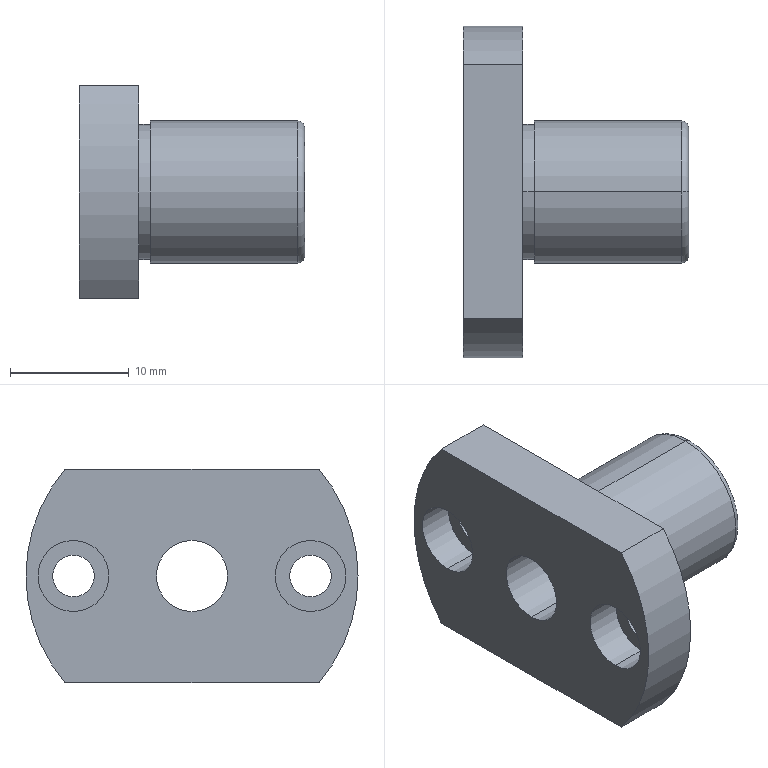Part | STEP file | 11-LHFC6C11_LHFC6 | 1 solid | 26 faces | box 19 x 28 x 18 mm | volume 3154 mm3 | cylinder 16 | plane 8 | torus 2 | commonest cylinder face diameters 6 x6 3.5 x4 11.4 x2 12 x2 28 x2
STEP:
#1=CARTESIAN_POINT('',(5.,-10.,-1.75));
#2=VERTEX_POINT('',#1);
#3=CARTESIAN_POINT('',(5.,-10.,1.75));
#4=VERTEX_POINT('',#3);
#5=CARTESIAN_POINT('',(5.,-10.,0.));
#6=DIRECTION('',(-1.,0.,0.));
#7=DIRECTION('',(0.,0.,1.));
#8=AXIS2_PLACEMENT_3D('',#5,#6,#7);
#9=CIRCLE('',#8,1.75);
#10=EDGE_CURVE('',#2,#4,#9,.T.);
#11=ORIENTED_EDGE('',*,*,#10,.F.);
#12=CARTESIAN_POINT('',(3.1,-10.,-1.75));
#13=VERTEX_POINT('',#12);
#14=CARTESIAN_POINT('',(5.,-10.,-1.75));
#15=DIRECTION('',(-1.,0.,0.));
#16=VECTOR('',#15,1000.);
#17=LINE('',#14,#16);
#18=EDGE_CURVE('',#2,#13,#17,.T.);
#19=ORIENTED_EDGE('',*,*,#18,.T.);
#20=CARTESIAN_POINT('',(3.1,-10.,1.75));
#21=VERTEX_POINT('',#20);
#22=CARTESIAN_POINT('',(3.1,-10.,0.));
#23=DIRECTION('',(-1.,0.,0.));
#24=DIRECTION('',(0.,0.,1.));
#25=AXIS2_PLACEMENT_3D('',#22,#23,#24);
#26=CIRCLE('',#25,1.75);
#27=EDGE_CURVE('',#13,#21,#26,.T.);
#28=ORIENTED_EDGE('',*,*,#27,.T.);
#29=CARTESIAN_POINT('',(5.,-10.,1.75));
#30=DIRECTION('',(-1.,0.,0.));
#31=VECTOR('',#30,1000.);
#32=LINE('',#29,#31);
#33=EDGE_CURVE('',#4,#21,#32,.T.);
#34=ORIENTED_EDGE('',*,*,#33,.F.);
#35=EDGE_LOOP('',(#11,#19,#28,#34));
#36=FACE_OUTER_BOUND('',#35,.T.);
#37=CARTESIAN_POINT('',(5.,-10.,0.));
#38=DIRECTION('',(-1.,0.,0.));
#39=DIRECTION('',(0.,0.,1.));
#40=AXIS2_PLACEMENT_3D('',#37,#38,#39);
#41=CYLINDRICAL_SURFACE('',#40,1.75);
#42=ADVANCED_FACE('',(#36),#41,.F.);
#43=CARTESIAN_POINT('',(3.1,-10.,-3.));
#44=VERTEX_POINT('',#43);
#45=CARTESIAN_POINT('',(3.1,-10.,3.));
#46=VERTEX_POINT('',#45);
#47=CARTESIAN_POINT('',(3.1,-10.,0.));
#48=DIRECTION('',(-1.,0.,0.));
#49=DIRECTION('',(0.,0.,1.));
#50=AXIS2_PLACEMENT_3D('',#47,#48,#49);
#51=CIRCLE('',#50,3.);
#52=EDGE_CURVE('',#44,#46,#51,.T.);
#53=ORIENTED_EDGE('',*,*,#52,.F.);
#54=CARTESIAN_POINT('',(0.,-10.,-3.));
#55=VERTEX_POINT('',#54);
#56=CARTESIAN_POINT('',(5.,-10.,-3.));
#57=DIRECTION('',(-1.,0.,0.));
#58=VECTOR('',#57,1000.);
#59=LINE('',#56,#58);
#60=EDGE_CURVE('',#44,#55,#59,.T.);
#61=ORIENTED_EDGE('',*,*,#60,.T.);
#62=CARTESIAN_POINT('',(0.,-10.,3.));
#63=VERTEX_POINT('',#62);
#64=CARTESIAN_POINT('',(0.,-10.,0.));
#65=DIRECTION('',(-1.,0.,0.));
#66=DIRECTION('',(0.,0.,1.));
#67=AXIS2_PLACEMENT_3D('',#64,#65,#66);
#68=CIRCLE('',#67,3.);
#69=EDGE_CURVE('',#55,#63,#68,.T.);
#70=ORIENTED_EDGE('',*,*,#69,.T.);
#71=CARTESIAN_POINT('',(5.,-10.,3.));
#72=DIRECTION('',(-1.,0.,0.));
#73=VECTOR('',#72,1000.);
#74=LINE('',#71,#73);
#75=EDGE_CURVE('',#46,#63,#74,.T.);
#76=ORIENTED_EDGE('',*,*,#75,.F.);
#77=EDGE_LOOP('',(#53,#61,#70,#76));
#78=FACE_OUTER_BOUND('',#77,.T.);
#79=CARTESIAN_POINT('',(5.,-10.,0.));
#80=DIRECTION('',(-1.,0.,0.));
#81=DIRECTION('',(0.,0.,1.));
#82=AXIS2_PLACEMENT_3D('',#79,#80,#81);
#83=CYLINDRICAL_SURFACE('',#82,3.);
#84=ADVANCED_FACE('',(#78),#83,.F.);
#85=CARTESIAN_POINT('',(5.,10.,-1.75));
#86=VERTEX_POINT('',#85);
#87=CARTESIAN_POINT('',(5.,10.,1.75));
#88=VERTEX_POINT('',#87);
#89=CARTESIAN_POINT('',(5.,10.,0.));
#90=DIRECTION('',(-1.,0.,0.));
#91=DIRECTION('',(0.,0.,1.));
#92=AXIS2_PLACEMENT_3D('',#89,#90,#91);
#93=CIRCLE('',#92,1.75);
#94=EDGE_CURVE('',#86,#88,#93,.T.);
#95=ORIENTED_EDGE('',*,*,#94,.F.);
#96=CARTESIAN_POINT('',(3.1,10.,-1.75));
#97=VERTEX_POINT('',#96);
#98=CARTESIAN_POINT('',(5.,10.,-1.75));
#99=DIRECTION('',(-1.,0.,0.));
#100=VECTOR('',#99,1000.);
#101=LINE('',#98,#100);
#102=EDGE_CURVE('',#86,#97,#101,.T.);
#103=ORIENTED_EDGE('',*,*,#102,.T.);
#104=CARTESIAN_POINT('',(3.1,10.,1.75));
#105=VERTEX_POINT('',#104);
#106=CARTESIAN_POINT('',(3.1,10.,0.));
#107=DIRECTION('',(-1.,0.,0.));
#108=DIRECTION('',(0.,0.,1.));
#109=AXIS2_PLACEMENT_3D('',#106,#107,#108);
#110=CIRCLE('',#109,1.75);
#111=EDGE_CURVE('',#97,#105,#110,.T.);
#112=ORIENTED_EDGE('',*,*,#111,.T.);
#113=CARTESIAN_POINT('',(5.,10.,1.75));
#114=DIRECTION('',(-1.,0.,0.));
#115=VECTOR('',#114,1000.);
#116=LINE('',#113,#115);
#117=EDGE_CURVE('',#88,#105,#116,.T.);
#118=ORIENTED_EDGE('',*,*,#117,.F.);
#119=EDGE_LOOP('',(#95,#103,#112,#118));
#120=FACE_OUTER_BOUND('',#119,.T.);
#121=CARTESIAN_POINT('',(5.,10.,0.));
#122=DIRECTION('',(-1.,0.,0.));
#123=DIRECTION('',(0.,0.,1.));
#124=AXIS2_PLACEMENT_3D('',#121,#122,#123);
#125=CYLINDRICAL_SURFACE('',#124,1.75);
#126=ADVANCED_FACE('',(#120),#125,.F.);
#127=CARTESIAN_POINT('',(3.1,10.,-3.));
#128=VERTEX_POINT('',#127);
#129=CARTESIAN_POINT('',(3.1,10.,3.));
#130=VERTEX_POINT('',#129);
#131=CARTESIAN_POINT('',(3.1,10.,0.));
#132=DIRECTION('',(-1.,0.,0.));
#133=DIRECTION('',(0.,0.,1.));
#134=AXIS2_PLACEMENT_3D('',#131,#132,#133);
#135=CIRCLE('',#134,3.);
#136=EDGE_CURVE('',#128,#130,#135,.T.);
#137=ORIENTED_EDGE('',*,*,#136,.F.);
#138=CARTESIAN_POINT('',(0.,10.,-3.));
#139=VERTEX_POINT('',#138);
#140=CARTESIAN_POINT('',(5.,10.,-3.));
#141=DIRECTION('',(-1.,0.,0.));
#142=VECTOR('',#141,1000.);
#143=LINE('',#140,#142);
#144=EDGE_CURVE('',#128,#139,#143,.T.);
#145=ORIENTED_EDGE('',*,*,#144,.T.);
#146=CARTESIAN_POINT('',(0.,10.,3.));
#147=VERTEX_POINT('',#146);
#148=CARTESIAN_POINT('',(0.,10.,0.));
#149=DIRECTION('',(-1.,0.,0.));
#150=DIRECTION('',(0.,0.,1.));
#151=AXIS2_PLACEMENT_3D('',#148,#149,#150);
#152=CIRCLE('',#151,3.);
#153=EDGE_CURVE('',#139,#147,#152,.T.);
#154=ORIENTED_EDGE('',*,*,#153,.T.);
#155=CARTESIAN_POINT('',(5.,10.,3.));
#156=DIRECTION('',(-1.,0.,0.));
#157=VECTOR('',#156,1000.);
#158=LINE('',#155,#157);
#159=EDGE_CURVE('',#130,#147,#158,.T.);
#160=ORIENTED_EDGE('',*,*,#159,.F.);
#161=EDGE_LOOP('',(#137,#145,#154,#160));
#162=FACE_OUTER_BOUND('',#161,.T.);
#163=CARTESIAN_POINT('',(5.,10.,0.));
#164=DIRECTION('',(-1.,0.,0.));
#165=DIRECTION('',(0.,0.,1.));
#166=AXIS2_PLACEMENT_3D('',#163,#164,#165);
#167=CYLINDRICAL_SURFACE('',#166,3.);
#168=ADVANCED_FACE('',(#162),#167,.F.);
#169=CARTESIAN_POINT('',(6.,0.,5.7));
#170=VERTEX_POINT('',#169);
#171=CARTESIAN_POINT('',(6.,0.,-5.7));
#172=VERTEX_POINT('',#171);
#173=CARTESIAN_POINT('',(6.,0.,0.));
#174=DIRECTION('',(-1.,0.,0.));
#175=DIRECTION('',(0.,0.,1.));
#176=AXIS2_PLACEMENT_3D('',#173,#174,#175);
#177=CIRCLE('',#176,5.7);
#178=EDGE_CURVE('',#170,#172,#177,.T.);
#179=ORIENTED_EDGE('',*,*,#178,.T.);
#180=CARTESIAN_POINT('',(5.,0.,-5.7));
#181=VERTEX_POINT('',#180);
#182=CARTESIAN_POINT('',(19.,0.,-5.7));
#183=DIRECTION('',(-1.,0.,0.));
#184=VECTOR('',#183,1000.);
#185=LINE('',#182,#184);
#186=EDGE_CURVE('',#172,#181,#185,.T.);
#187=ORIENTED_EDGE('',*,*,#186,.T.);
#188=CARTESIAN_POINT('',(5.,0.,5.7));
#189=VERTEX_POINT('',#188);
#190=CARTESIAN_POINT('',(5.,0.,0.));
#191=DIRECTION('',(-1.,0.,0.));
#192=DIRECTION('',(0.,0.,1.));
#193=AXIS2_PLACEMENT_3D('',#190,#191,#192);
#194=CIRCLE('',#193,5.7);
#195=EDGE_CURVE('',#189,#181,#194,.T.);
#196=ORIENTED_EDGE('',*,*,#195,.F.);
#197=CARTESIAN_POINT('',(19.,0.,5.7));
#198=DIRECTION('',(-1.,0.,0.));
#199=VECTOR('',#198,1000.);
#200=LINE('',#197,#199);
#201=EDGE_CURVE('',#170,#189,#200,.T.);
#202=ORIENTED_EDGE('',*,*,#201,.F.);
#203=EDGE_LOOP('',(#179,#187,#196,#202));
#204=FACE_OUTER_BOUND('',#203,.T.);
#205=CARTESIAN_POINT('',(19.,0.,0.));
#206=DIRECTION('',(-1.,0.,0.));
#207=DIRECTION('',(0.,0.,1.));
#208=AXIS2_PLACEMENT_3D('',#205,#206,#207);
#209=CYLINDRICAL_SURFACE('',#208,5.7);
#210=ADVANCED_FACE('',(#204),#209,.T.);
#211=CARTESIAN_POINT('',(18.4,0.,6.));
#212=VERTEX_POINT('',#211);
#213=CARTESIAN_POINT('',(18.4,0.,-6.));
#214=VERTEX_POINT('',#213);
#215=CARTESIAN_POINT('',(18.4,0.,0.));
#216=DIRECTION('',(-1.,0.,0.));
#217=DIRECTION('',(0.,0.,1.));
#218=AXIS2_PLACEMENT_3D('',#215,#216,#217);
#219=CIRCLE('',#218,6.);
#220=EDGE_CURVE('',#212,#214,#219,.T.);
#221=ORIENTED_EDGE('',*,*,#220,.T.);
#222=CARTESIAN_POINT('',(6.,0.,-6.));
#223=VERTEX_POINT('',#222);
#224=CARTESIAN_POINT('',(19.,0.,-6.));
#225=DIRECTION('',(-1.,0.,0.));
#226=VECTOR('',#225,1000.);
#227=LINE('',#224,#226);
#228=EDGE_CURVE('',#214,#223,#227,.T.);
#229=ORIENTED_EDGE('',*,*,#228,.T.);
#230=CARTESIAN_POINT('',(6.,0.,6.));
#231=VERTEX_POINT('',#230);
#232=CARTESIAN_POINT('',(6.,0.,0.));
#233=DIRECTION('',(-1.,0.,0.));
#234=DIRECTION('',(0.,0.,1.));
#235=AXIS2_PLACEMENT_3D('',#232,#233,#234);
#236=CIRCLE('',#235,6.);
#237=EDGE_CURVE('',#231,#223,#236,.T.);
#238=ORIENTED_EDGE('',*,*,#237,.F.);
#239=CARTESIAN_POINT('',(19.,0.,6.));
#240=DIRECTION('',(-1.,0.,0.));
#241=VECTOR('',#240,1000.);
#242=LINE('',#239,#241);
#243=EDGE_CURVE('',#212,#231,#242,.T.);
#244=ORIENTED_EDGE('',*,*,#243,.F.);
#245=EDGE_LOOP('',(#221,#229,#238,#244));
#246=FACE_OUTER_BOUND('',#245,.T.);
#247=CARTESIAN_POINT('',(19.,0.,0.));
#248=DIRECTION('',(-1.,0.,0.));
#249=DIRECTION('',(0.,0.,1.));
#250=AXIS2_PLACEMENT_3D('',#247,#248,#249);
#251=CYLINDRICAL_SURFACE('',#250,6.);
#252=ADVANCED_FACE('',(#246),#251,.T.);
#253=CARTESIAN_POINT('',(19.,0.,5.4));
#254=VERTEX_POINT('',#253);
#255=CARTESIAN_POINT('',(19.,0.,-5.4));
#256=VERTEX_POINT('',#255);
#257=CARTESIAN_POINT('',(19.,0.,0.));
#258=DIRECTION('',(-1.,0.,0.));
#259=DIRECTION('',(0.,0.,1.));
#260=AXIS2_PLACEMENT_3D('',#257,#258,#259);
#261=CIRCLE('',#260,5.4);
#262=EDGE_CURVE('',#254,#256,#261,.T.);
#263=ORIENTED_EDGE('',*,*,#262,.T.);
#264=CARTESIAN_POINT('',(18.4,0.,-5.4));
#265=DIRECTION('',(0.,1.,0.));
#266=DIRECTION('',(0.,0.,1.));
#267=AXIS2_PLACEMENT_3D('',#264,#265,#266);
#268=CIRCLE('',#267,0.6);
#269=EDGE_CURVE('',#256,#214,#268,.T.);
#270=ORIENTED_EDGE('',*,*,#269,.T.);
#271=ORIENTED_EDGE('',*,*,#220,.F.);
#272=CARTESIAN_POINT('',(18.4,0.,5.4));
#273=DIRECTION('',(0.,-1.,0.));
#274=DIRECTION('',(0.,0.,-1.));
#275=AXIS2_PLACEMENT_3D('',#272,#273,#274);
#276=CIRCLE('',#275,0.6);
#277=EDGE_CURVE('',#254,#212,#276,.T.);
#278=ORIENTED_EDGE('',*,*,#277,.F.);
#279=EDGE_LOOP('',(#263,#270,#271,#278));
#280=FACE_OUTER_BOUND('',#279,.T.);
#281=CARTESIAN_POINT('',(18.4,0.,0.));
#282=DIRECTION('',(-1.,0.,0.));
#283=DIRECTION('',(0.,0.,1.));
#284=AXIS2_PLACEMENT_3D('',#281,#282,#283);
#285=TOROIDAL_SURFACE('',#284,5.4,0.6);
#286=ADVANCED_FACE('',(#280),#285,.T.);
#287=CARTESIAN_POINT('',(19.,0.,-3.));
#288=VERTEX_POINT('',#287);
#289=CARTESIAN_POINT('',(19.,0.,3.));
#290=VERTEX_POINT('',#289);
#291=CARTESIAN_POINT('',(19.,0.,0.));
#292=DIRECTION('',(-1.,0.,0.));
#293=DIRECTION('',(0.,0.,1.));
#294=AXIS2_PLACEMENT_3D('',#291,#292,#293);
#295=CIRCLE('',#294,3.);
#296=EDGE_CURVE('',#288,#290,#295,.T.);
#297=ORIENTED_EDGE('',*,*,#296,.F.);
#298=CARTESIAN_POINT('',(0.,0.,-3.));
#299=VERTEX_POINT('',#298);
#300=CARTESIAN_POINT('',(19.,0.,-3.));
#301=DIRECTION('',(-1.,0.,0.));
#302=VECTOR('',#301,1000.);
#303=LINE('',#300,#302);
#304=EDGE_CURVE('',#288,#299,#303,.T.);
#305=ORIENTED_EDGE('',*,*,#304,.T.);
#306=CARTESIAN_POINT('',(0.,0.,3.));
#307=VERTEX_POINT('',#306);
#308=CARTESIAN_POINT('',(0.,0.,0.));
#309=DIRECTION('',(-1.,0.,0.));
#310=DIRECTION('',(0.,0.,1.));
#311=AXIS2_PLACEMENT_3D('',#308,#309,#310);
#312=CIRCLE('',#311,3.);
#313=EDGE_CURVE('',#299,#307,#312,.T.);
#314=ORIENTED_EDGE('',*,*,#313,.T.);
#315=CARTESIAN_POINT('',(19.,0.,3.));
#316=DIRECTION('',(-1.,0.,0.));
#317=VECTOR('',#316,1000.);
#318=LINE('',#315,#317);
#319=EDGE_CURVE('',#290,#307,#318,.T.);
#320=ORIENTED_EDGE('',*,*,#319,.F.);
#321=EDGE_LOOP('',(#297,#305,#314,#320));
#322=FACE_OUTER_BOUND('',#321,.T.);
#323=CARTESIAN_POINT('',(19.,0.,0.));
#324=DIRECTION('',(-1.,0.,0.));
#325=DIRECTION('',(0.,0.,1.));
#326=AXIS2_PLACEMENT_3D('',#323,#324,#325);
#327=CYLINDRICAL_SURFACE('',#326,3.);
#328=ADVANCED_FACE('',(#322),#327,.F.);
#329=CARTESIAN_POINT('',(5.,10.724,9.));
#330=VERTEX_POINT('',#329);
#331=CARTESIAN_POINT('',(5.,10.724,-9.));
#332=VERTEX_POINT('',#331);
#333=CARTESIAN_POINT('',(5.,0.,0.));
#334=DIRECTION('',(-1.,0.,0.));
#335=DIRECTION('',(0.,0.,1.));
#336=AXIS2_PLACEMENT_3D('',#333,#334,#335);
#337=CIRCLE('',#336,14.);
#338=EDGE_CURVE('',#330,#332,#337,.T.);
#339=ORIENTED_EDGE('',*,*,#338,.T.);
#340=CARTESIAN_POINT('',(0.,10.724,-9.));
#341=VERTEX_POINT('',#340);
#342=CARTESIAN_POINT('',(5.,10.724,-9.));
#343=DIRECTION('',(-1.,0.,0.));
#344=VECTOR('',#343,1000.);
#345=LINE('',#342,#344);
#346=EDGE_CURVE('',#332,#341,#345,.T.);
#347=ORIENTED_EDGE('',*,*,#346,.T.);
#348=CARTESIAN_POINT('',(0.,10.724,9.));
#349=VERTEX_POINT('',#348);
#350=CARTESIAN_POINT('',(0.,0.,0.));
#351=DIRECTION('',(-1.,0.,0.));
#352=DIRECTION('',(0.,0.,1.));
#353=AXIS2_PLACEMENT_3D('',#350,#351,#352);
#354=CIRCLE('',#353,14.);
#355=EDGE_CURVE('',#349,#341,#354,.T.);
#356=ORIENTED_EDGE('',*,*,#355,.F.);
#357=CARTESIAN_POINT('',(5.,10.724,9.));
#358=DIRECTION('',(-1.,0.,0.));
#359=VECTOR('',#358,1000.);
#360=LINE('',#357,#359);
#361=EDGE_CURVE('',#330,#349,#360,.T.);
#362=ORIENTED_EDGE('',*,*,#361,.F.);
#363=EDGE_LOOP('',(#339,#347,#356,#362));
#364=FACE_OUTER_BOUND('',#363,.T.);
#365=CARTESIAN_POINT('',(19.,0.,0.));
#366=DIRECTION('',(-1.,0.,0.));
#367=DIRECTION('',(0.,0.,1.));
#368=AXIS2_PLACEMENT_3D('',#365,#366,#367);
#369=CYLINDRICAL_SURFACE('',#368,14.);
#370=ADVANCED_FACE('',(#364),#369,.T.);
#371=CARTESIAN_POINT('',(0.,-10.724,-9.));
#372=VERTEX_POINT('',#371);
#373=CARTESIAN_POINT('',(0.,-10.724,9.));
#374=VERTEX_POINT('',#373);
#375=CARTESIAN_POINT('',(0.,0.,0.));
#376=DIRECTION('',(-1.,0.,0.));
#377=DIRECTION('',(0.,0.,1.));
#378=AXIS2_PLACEMENT_3D('',#375,#376,#377);
#379=CIRCLE('',#378,14.);
#380=EDGE_CURVE('',#372,#374,#379,.T.);
#381=ORIENTED_EDGE('',*,*,#380,.F.);
#382=CARTESIAN_POINT('',(5.,-10.724,-9.));
#383=VERTEX_POINT('',#382);
#384=CARTESIAN_POINT('',(5.,-10.724,-9.));
#385=DIRECTION('',(-1.,0.,0.));
#386=VECTOR('',#385,1000.);
#387=LINE('',#384,#386);
#388=EDGE_CURVE('',#383,#372,#387,.T.);
#389=ORIENTED_EDGE('',*,*,#388,.F.);
#390=CARTESIAN_POINT('',(5.,-10.724,9.));
#391=VERTEX_POINT('',#390);
#392=CARTESIAN_POINT('',(5.,0.,0.));
#393=DIRECTION('',(-1.,0.,0.));
#394=DIRECTION('',(0.,0.,1.));
#395=AXIS2_PLACEMENT_3D('',#392,#393,#394);
#396=CIRCLE('',#395,14.);
#397=EDGE_CURVE('',#383,#391,#396,.T.);
#398=ORIENTED_EDGE('',*,*,#397,.T.);
#399=CARTESIAN_POINT('',(5.,-10.724,9.));
#400=DIRECTION('',(-1.,0.,0.));
#401=VECTOR('',#400,1000.);
#402=LINE('',#399,#401);
#403=EDGE_CURVE('',#391,#374,#402,.T.);
#404=ORIENTED_EDGE('',*,*,#403,.T.);
#405=EDGE_LOOP('',(#381,#389,#398,#404));
#406=FACE_OUTER_BOUND('',#405,.T.);
#407=CARTESIAN_POINT('',(19.,0.,0.));
#408=DIRECTION('',(-1.,0.,0.));
#409=DIRECTION('',(0.,0.,1.));
#410=AXIS2_PLACEMENT_3D('',#407,#408,#409);
#411=CYLINDRICAL_SURFACE('',#410,14.);
#412=ADVANCED_FACE('',(#406),#411,.T.);
#413=CARTESIAN_POINT('',(0.,-10.,0.));
#414=DIRECTION('',(-1.,0.,0.));
#415=DIRECTION('',(0.,0.,1.));
#416=AXIS2_PLACEMENT_3D('',#413,#414,#415);
#417=CIRCLE('',#416,3.);
#418=EDGE_CURVE('',#63,#55,#417,.T.);
#419=ORIENTED_EDGE('',*,*,#418,.F.);
#420=ORIENTED_EDGE('',*,*,#69,.F.);
#421=EDGE_LOOP('',(#419,#420));
#422=FACE_BOUND('',#421,.T.);
#423=CARTESIAN_POINT('',(0.,10.,0.));
#424=DIRECTION('',(-1.,0.,0.));
#425=DIRECTION('',(0.,0.,1.));
#426=AXIS2_PLACEMENT_3D('',#423,#424,#425);
#427=CIRCLE('',#426,3.);
#428=EDGE_CURVE('',#147,#139,#427,.T.);
#429=ORIENTED_EDGE('',*,*,#428,.F.);
#430=ORIENTED_EDGE('',*,*,#153,.F.);
#431=EDGE_LOOP('',(#429,#430));
#432=FACE_BOUND('',#431,.T.);
#433=CARTESIAN_POINT('',(0.,0.,0.));
#434=DIRECTION('',(-1.,0.,0.));
#435=DIRECTION('',(0.,0.,1.));
#436=AXIS2_PLACEMENT_3D('',#433,#434,#435);
#437=CIRCLE('',#436,3.);
#438=EDGE_CURVE('',#307,#299,#437,.T.);
#439=ORIENTED_EDGE('',*,*,#438,.F.);
#440=ORIENTED_EDGE('',*,*,#313,.F.);
#441=EDGE_LOOP('',(#439,#440));
#442=FACE_BOUND('',#441,.T.);
#443=ORIENTED_EDGE('',*,*,#355,.T.);
#444=CARTESIAN_POINT('',(0.,-10.724,-9.));
#445=DIRECTION('',(0.,1.,0.));
#446=VECTOR('',#445,1000.);
#447=LINE('',#444,#446);
#448=EDGE_CURVE('',#372,#341,#447,.T.);
#449=ORIENTED_EDGE('',*,*,#448,.F.);
#450=ORIENTED_EDGE('',*,*,#380,.T.);
#451=CARTESIAN_POINT('',(0.,10.724,9.));
#452=DIRECTION('',(0.,-1.,0.));
#453=VECTOR('',#452,1000.);
#454=LINE('',#451,#453);
#455=EDGE_CURVE('',#349,#374,#454,.T.);
#456=ORIENTED_EDGE('',*,*,#455,.F.);
#457=EDGE_LOOP('',(#443,#449,#450,#456));
#458=FACE_OUTER_BOUND('',#457,.T.);
#459=CARTESIAN_POINT('',(0.,14.,0.));
#460=DIRECTION('',(1.,0.,0.));
#461=DIRECTION('',(0.,0.,-1.));
#462=AXIS2_PLACEMENT_3D('',#459,#460,#461);
#463=PLANE('',#462);
#464=ADVANCED_FACE('',(#422,#432,#442,#458),#463,.F.);
#465=ORIENTED_EDGE('',*,*,#304,.F.);
#466=CARTESIAN_POINT('',(19.,0.,0.));
#467=DIRECTION('',(-1.,0.,0.));
#468=DIRECTION('',(0.,0.,1.));
#469=AXIS2_PLACEMENT_3D('',#466,#467,#468);
#470=CIRCLE('',#469,3.);
#471=EDGE_CURVE('',#290,#288,#470,.T.);
#472=ORIENTED_EDGE('',*,*,#471,.F.);
#473=ORIENTED_EDGE('',*,*,#319,.T.);
#474=ORIENTED_EDGE('',*,*,#438,.T.);
#475=EDGE_LOOP('',(#465,#472,#473,#474));
#476=FACE_OUTER_BOUND('',#475,.T.);
#477=CARTESIAN_POINT('',(19.,0.,0.));
#478=DIRECTION('',(-1.,0.,0.));
#479=DIRECTION('',(0.,0.,1.));
#480=AXIS2_PLACEMENT_3D('',#477,#478,#479);
#481=CYLINDRICAL_SURFACE('',#480,3.);
#482=ADVANCED_FACE('',(#476),#481,.F.);
#483=ORIENTED_EDGE('',*,*,#262,.F.);
#484=CARTESIAN_POINT('',(19.,0.,0.));
#485=DIRECTION('',(-1.,0.,0.));
#486=DIRECTION('',(0.,0.,1.));
#487=AXIS2_PLACEMENT_3D('',#484,#485,#486);
#488=CIRCLE('',#487,5.4);
#489=EDGE_CURVE('',#256,#254,#488,.T.);
#490=ORIENTED_EDGE('',*,*,#489,.F.);
#491=EDGE_LOOP('',(#483,#490));
#492=FACE_OUTER_BOUND('',#491,.T.);
#493=ORIENTED_EDGE('',*,*,#471,.T.);
#494=ORIENTED_EDGE('',*,*,#296,.T.);
#495=EDGE_LOOP('',(#493,#494));
#496=FACE_BOUND('',#495,.T.);
#497=CARTESIAN_POINT('',(19.,3.,0.));
#498=DIRECTION('',(-1.,0.,0.));
#499=DIRECTION('',(0.,0.,1.));
#500=AXIS2_PLACEMENT_3D('',#497,#498,#499);
#501=PLANE('',#500);
#502=ADVANCED_FACE('',(#492,#496),#501,.F.);
#503=ORIENTED_EDGE('',*,*,#269,.F.);
#504=ORIENTED_EDGE('',*,*,#489,.T.);
#505=ORIENTED_EDGE('',*,*,#277,.T.);
#506=CARTESIAN_POINT('',(18.4,0.,0.));
#507=DIRECTION('',(-1.,0.,0.));
#508=DIRECTION('',(0.,0.,1.));
#509=AXIS2_PLACEMENT_3D('',#506,#507,#508);
#510=CIRCLE('',#509,6.);
#511=EDGE_CURVE('',#214,#212,#510,.T.);
#512=ORIENTED_EDGE('',*,*,#511,.F.);
#513=EDGE_LOOP('',(#503,#504,#505,#512));
#514=FACE_OUTER_BOUND('',#513,.T.);
#515=CARTESIAN_POINT('',(18.4,0.,0.));
#516=DIRECTION('',(-1.,0.,0.));
#517=DIRECTION('',(0.,0.,1.));
#518=AXIS2_PLACEMENT_3D('',#515,#516,#517);
#519=TOROIDAL_SURFACE('',#518,5.4,0.6);
#520=ADVANCED_FACE('',(#514),#519,.T.);
#521=ORIENTED_EDGE('',*,*,#228,.F.);
#522=ORIENTED_EDGE('',*,*,#511,.T.);
#523=ORIENTED_EDGE('',*,*,#243,.T.);
#524=CARTESIAN_POINT('',(6.,0.,0.));
#525=DIRECTION('',(-1.,0.,0.));
#526=DIRECTION('',(0.,0.,1.));
#527=AXIS2_PLACEMENT_3D('',#524,#525,#526);
#528=CIRCLE('',#527,6.);
#529=EDGE_CURVE('',#223,#231,#528,.T.);
#530=ORIENTED_EDGE('',*,*,#529,.F.);
#531=EDGE_LOOP('',(#521,#522,#523,#530));
#532=FACE_OUTER_BOUND('',#531,.T.);
#533=CARTESIAN_POINT('',(19.,0.,0.));
#534=DIRECTION('',(-1.,0.,0.));
#535=DIRECTION('',(0.,0.,1.));
#536=AXIS2_PLACEMENT_3D('',#533,#534,#535);
#537=CYLINDRICAL_SURFACE('',#536,6.);
#538=ADVANCED_FACE('',(#532),#537,.T.);
#539=ORIENTED_EDGE('',*,*,#178,.F.);
#540=CARTESIAN_POINT('',(6.,0.,0.));
#541=DIRECTION('',(-1.,0.,0.));
#542=DIRECTION('',(0.,0.,1.));
#543=AXIS2_PLACEMENT_3D('',#540,#541,#542);
#544=CIRCLE('',#543,5.7);
#545=EDGE_CURVE('',#172,#170,#544,.T.);
#546=ORIENTED_EDGE('',*,*,#545,.F.);
#547=EDGE_LOOP('',(#539,#546));
#548=FACE_BOUND('',#547,.T.);
#549=ORIENTED_EDGE('',*,*,#237,.T.);
#550=ORIENTED_EDGE('',*,*,#529,.T.);
#551=EDGE_LOOP('',(#549,#550));
#552=FACE_OUTER_BOUND('',#551,.T.);
#553=CARTESIAN_POINT('',(6.,6.,0.));
#554=DIRECTION('',(1.,0.,0.));
#555=DIRECTION('',(0.,0.,-1.));
#556=AXIS2_PLACEMENT_3D('',#553,#554,#555);
#557=PLANE('',#556);
#558=ADVANCED_FACE('',(#548,#552),#557,.F.);
#559=ORIENTED_EDGE('',*,*,#186,.F.);
#560=ORIENTED_EDGE('',*,*,#545,.T.);
#561=ORIENTED_EDGE('',*,*,#201,.T.);
#562=CARTESIAN_POINT('',(5.,0.,0.));
#563=DIRECTION('',(-1.,0.,0.));
#564=DIRECTION('',(0.,0.,1.));
#565=AXIS2_PLACEMENT_3D('',#562,#563,#564);
#566=CIRCLE('',#565,5.7);
#567=EDGE_CURVE('',#181,#189,#566,.T.);
#568=ORIENTED_EDGE('',*,*,#567,.F.);
#569=EDGE_LOOP('',(#559,#560,#561,#568));
#570=FACE_OUTER_BOUND('',#569,.T.);
#571=CARTESIAN_POINT('',(19.,0.,0.));
#572=DIRECTION('',(-1.,0.,0.));
#573=DIRECTION('',(0.,0.,1.));
#574=AXIS2_PLACEMENT_3D('',#571,#572,#573);
#575=CYLINDRICAL_SURFACE('',#574,5.7);
#576=ADVANCED_FACE('',(#570),#575,.T.);
#577=CARTESIAN_POINT('',(5.,-10.,0.));
#578=DIRECTION('',(-1.,0.,0.));
#579=DIRECTION('',(0.,0.,1.));
#580=AXIS2_PLACEMENT_3D('',#577,#578,#579);
#581=CIRCLE('',#580,1.75);
#582=EDGE_CURVE('',#4,#2,#581,.T.);
#583=ORIENTED_EDGE('',*,*,#582,.T.);
#584=ORIENTED_EDGE('',*,*,#10,.T.);
#585=EDGE_LOOP('',(#583,#584));
#586=FACE_BOUND('',#585,.T.);
#587=CARTESIAN_POINT('',(5.,10.,0.));
#588=DIRECTION('',(-1.,0.,0.));
#589=DIRECTION('',(0.,0.,1.));
#590=AXIS2_PLACEMENT_3D('',#587,#588,#589);
#591=CIRCLE('',#590,1.75);
#592=EDGE_CURVE('',#88,#86,#591,.T.);
#593=ORIENTED_EDGE('',*,*,#592,.T.);
#594=ORIENTED_EDGE('',*,*,#94,.T.);
#595=EDGE_LOOP('',(#593,#594));
#596=FACE_BOUND('',#595,.T.);
#597=ORIENTED_EDGE('',*,*,#397,.F.);
#598=CARTESIAN_POINT('',(5.,-10.724,-9.));
#599=DIRECTION('',(0.,1.,0.));
#600=VECTOR('',#599,1000.);
#601=LINE('',#598,#600);
#602=EDGE_CURVE('',#383,#332,#601,.T.);
#603=ORIENTED_EDGE('',*,*,#602,.T.);
#604=ORIENTED_EDGE('',*,*,#338,.F.);
#605=CARTESIAN_POINT('',(5.,10.724,9.));
#606=DIRECTION('',(0.,-1.,0.));
#607=VECTOR('',#606,1000.);
#608=LINE('',#605,#607);
#609=EDGE_CURVE('',#330,#391,#608,.T.);
#610=ORIENTED_EDGE('',*,*,#609,.T.);
#611=EDGE_LOOP('',(#597,#603,#604,#610));
#612=FACE_OUTER_BOUND('',#611,.T.);
#613=ORIENTED_EDGE('',*,*,#195,.T.);
#614=ORIENTED_EDGE('',*,*,#567,.T.);
#615=EDGE_LOOP('',(#613,#614));
#616=FACE_BOUND('',#615,.T.);
#617=CARTESIAN_POINT('',(5.,5.7,0.));
#618=DIRECTION('',(-1.,0.,0.));
#619=DIRECTION('',(0.,0.,1.));
#620=AXIS2_PLACEMENT_3D('',#617,#618,#619);
#621=PLANE('',#620);
#622=ADVANCED_FACE('',(#586,#596,#612,#616),#621,.F.);
#623=ORIENTED_EDGE('',*,*,#455,.T.);
#624=ORIENTED_EDGE('',*,*,#403,.F.);
#625=ORIENTED_EDGE('',*,*,#609,.F.);
#626=ORIENTED_EDGE('',*,*,#361,.T.);
#627=EDGE_LOOP('',(#623,#624,#625,#626));
#628=FACE_OUTER_BOUND('',#627,.T.);
#629=CARTESIAN_POINT('',(5.,10.724,9.));
#630=DIRECTION('',(0.,0.,-1.));
#631=DIRECTION('',(-1.,0.,0.));
#632=AXIS2_PLACEMENT_3D('',#629,#630,#631);
#633=PLANE('',#632);
#634=ADVANCED_FACE('',(#628),#633,.F.);
#635=ORIENTED_EDGE('',*,*,#448,.T.);
#636=ORIENTED_EDGE('',*,*,#346,.F.);
#637=ORIENTED_EDGE('',*,*,#602,.F.);
#638=ORIENTED_EDGE('',*,*,#388,.T.);
#639=EDGE_LOOP('',(#635,#636,#637,#638));
#640=FACE_OUTER_BOUND('',#639,.T.);
#641=CARTESIAN_POINT('',(5.,-10.724,-9.));
#642=DIRECTION('',(0.,0.,1.));
#643=DIRECTION('',(1.,0.,0.));
#644=AXIS2_PLACEMENT_3D('',#641,#642,#643);
#645=PLANE('',#644);
#646=ADVANCED_FACE('',(#640),#645,.F.);
#647=ORIENTED_EDGE('',*,*,#144,.F.);
#648=CARTESIAN_POINT('',(3.1,10.,0.));
#649=DIRECTION('',(-1.,0.,0.));
#650=DIRECTION('',(0.,0.,1.));
#651=AXIS2_PLACEMENT_3D('',#648,#649,#650);
#652=CIRCLE('',#651,3.);
#653=EDGE_CURVE('',#130,#128,#652,.T.);
#654=ORIENTED_EDGE('',*,*,#653,.F.);
#655=ORIENTED_EDGE('',*,*,#159,.T.);
#656=ORIENTED_EDGE('',*,*,#428,.T.);
#657=EDGE_LOOP('',(#647,#654,#655,#656));
#658=FACE_OUTER_BOUND('',#657,.T.);
#659=CARTESIAN_POINT('',(5.,10.,0.));
#660=DIRECTION('',(-1.,0.,0.));
#661=DIRECTION('',(0.,0.,1.));
#662=AXIS2_PLACEMENT_3D('',#659,#660,#661);
#663=CYLINDRICAL_SURFACE('',#662,3.);
#664=ADVANCED_FACE('',(#658),#663,.F.);
#665=ORIENTED_EDGE('',*,*,#653,.T.);
#666=ORIENTED_EDGE('',*,*,#136,.T.);
#667=EDGE_LOOP('',(#665,#666));
#668=FACE_OUTER_BOUND('',#667,.T.);
#669=CARTESIAN_POINT('',(3.1,10.,0.));
#670=DIRECTION('',(-1.,0.,0.));
#671=DIRECTION('',(0.,0.,1.));
#672=AXIS2_PLACEMENT_3D('',#669,#670,#671);
#673=CIRCLE('',#672,1.75);
#674=EDGE_CURVE('',#105,#97,#673,.T.);
#675=ORIENTED_EDGE('',*,*,#674,.F.);
#676=ORIENTED_EDGE('',*,*,#111,.F.);
#677=EDGE_LOOP('',(#675,#676));
#678=FACE_BOUND('',#677,.T.);
#679=CARTESIAN_POINT('',(3.1,13.,0.));
#680=DIRECTION('',(-1.,0.,0.));
#681=DIRECTION('',(0.,0.,1.));
#682=AXIS2_PLACEMENT_3D('',#679,#680,#681);
#683=PLANE('',#682);
#684=ADVANCED_FACE('',(#668,#678),#683,.T.);
#685=ORIENTED_EDGE('',*,*,#102,.F.);
#686=ORIENTED_EDGE('',*,*,#592,.F.);
#687=ORIENTED_EDGE('',*,*,#117,.T.);
#688=ORIENTED_EDGE('',*,*,#674,.T.);
#689=EDGE_LOOP('',(#685,#686,#687,#688));
#690=FACE_OUTER_BOUND('',#689,.T.);
#691=CARTESIAN_POINT('',(5.,10.,0.));
#692=DIRECTION('',(-1.,0.,0.));
#693=DIRECTION('',(0.,0.,1.));
#694=AXIS2_PLACEMENT_3D('',#691,#692,#693);
#695=CYLINDRICAL_SURFACE('',#694,1.75);
#696=ADVANCED_FACE('',(#690),#695,.F.);
#697=ORIENTED_EDGE('',*,*,#60,.F.);
#698=CARTESIAN_POINT('',(3.1,-10.,0.));
#699=DIRECTION('',(-1.,0.,0.));
#700=DIRECTION('',(0.,0.,1.));
#701=AXIS2_PLACEMENT_3D('',#698,#699,#700);
#702=CIRCLE('',#701,3.);
#703=EDGE_CURVE('',#46,#44,#702,.T.);
#704=ORIENTED_EDGE('',*,*,#703,.F.);
#705=ORIENTED_EDGE('',*,*,#75,.T.);
#706=ORIENTED_EDGE('',*,*,#418,.T.);
#707=EDGE_LOOP('',(#697,#704,#705,#706));
#708=FACE_OUTER_BOUND('',#707,.T.);
#709=CARTESIAN_POINT('',(5.,-10.,0.));
#710=DIRECTION('',(-1.,0.,0.));
#711=DIRECTION('',(0.,0.,1.));
#712=AXIS2_PLACEMENT_3D('',#709,#710,#711);
#713=CYLINDRICAL_SURFACE('',#712,3.);
#714=ADVANCED_FACE('',(#708),#713,.F.);
#715=ORIENTED_EDGE('',*,*,#703,.T.);
#716=ORIENTED_EDGE('',*,*,#52,.T.);
#717=EDGE_LOOP('',(#715,#716));
#718=FACE_OUTER_BOUND('',#717,.T.);
#719=CARTESIAN_POINT('',(3.1,-10.,0.));
#720=DIRECTION('',(-1.,0.,0.));
#721=DIRECTION('',(0.,0.,1.));
#722=AXIS2_PLACEMENT_3D('',#719,#720,#721);
#723=CIRCLE('',#722,1.75);
#724=EDGE_CURVE('',#21,#13,#723,.T.);
#725=ORIENTED_EDGE('',*,*,#724,.F.);
#726=ORIENTED_EDGE('',*,*,#27,.F.);
#727=EDGE_LOOP('',(#725,#726));
#728=FACE_BOUND('',#727,.T.);
#729=CARTESIAN_POINT('',(3.1,-7.,0.));
#730=DIRECTION('',(-1.,0.,0.));
#731=DIRECTION('',(0.,0.,1.));
#732=AXIS2_PLACEMENT_3D('',#729,#730,#731);
#733=PLANE('',#732);
#734=ADVANCED_FACE('',(#718,#728),#733,.T.);
#735=ORIENTED_EDGE('',*,*,#18,.F.);
#736=ORIENTED_EDGE('',*,*,#582,.F.);
#737=ORIENTED_EDGE('',*,*,#33,.T.);
#738=ORIENTED_EDGE('',*,*,#724,.T.);
#739=EDGE_LOOP('',(#735,#736,#737,#738));
#740=FACE_OUTER_BOUND('',#739,.T.);
#741=CARTESIAN_POINT('',(5.,-10.,0.));
#742=DIRECTION('',(-1.,0.,0.));
#743=DIRECTION('',(0.,0.,1.));
#744=AXIS2_PLACEMENT_3D('',#741,#742,#743);
#745=CYLINDRICAL_SURFACE('',#744,1.75);
#746=ADVANCED_FACE('',(#740),#745,.F.);
#747=CLOSED_SHELL('',(#42,#84,#126,#168,#210,#252,#286,#328,#370,#412,#464,#482,#502,#520,#538,#558,#576,#622,#634,#646,#664,#684,#696,#714,#734,#746));
#748=MANIFOLD_SOLID_BREP('',#747);
#749=CARTESIAN_POINT('',(0.,0.,0.));
#750=DIRECTION('',(0.,0.,1.));
#751=DIRECTION('',(1.,0.,0.));
#752=AXIS2_PLACEMENT_3D('',#749,#750,#751);
#753=(LENGTH_UNIT()NAMED_UNIT(*)SI_UNIT(.MILLI.,.METRE.));
#754=UNCERTAINTY_MEASURE_WITH_UNIT(LENGTH_MEASURE(0.00001),#753,'','');
#755=(NAMED_UNIT(*)PLANE_ANGLE_UNIT()SI_UNIT($,.RADIAN.));
#756=(NAMED_UNIT(*)SI_UNIT($,.STERADIAN.)SOLID_ANGLE_UNIT());
#757=(GEOMETRIC_REPRESENTATION_CONTEXT(3)GLOBAL_UNCERTAINTY_ASSIGNED_CONTEXT((#754))GLOBAL_UNIT_ASSIGNED_CONTEXT((#753,#755,#756))REPRESENTATION_CONTEXT('',''));
#758=ADVANCED_BREP_SHAPE_REPRESENTATION('',(#748,#752),#757);